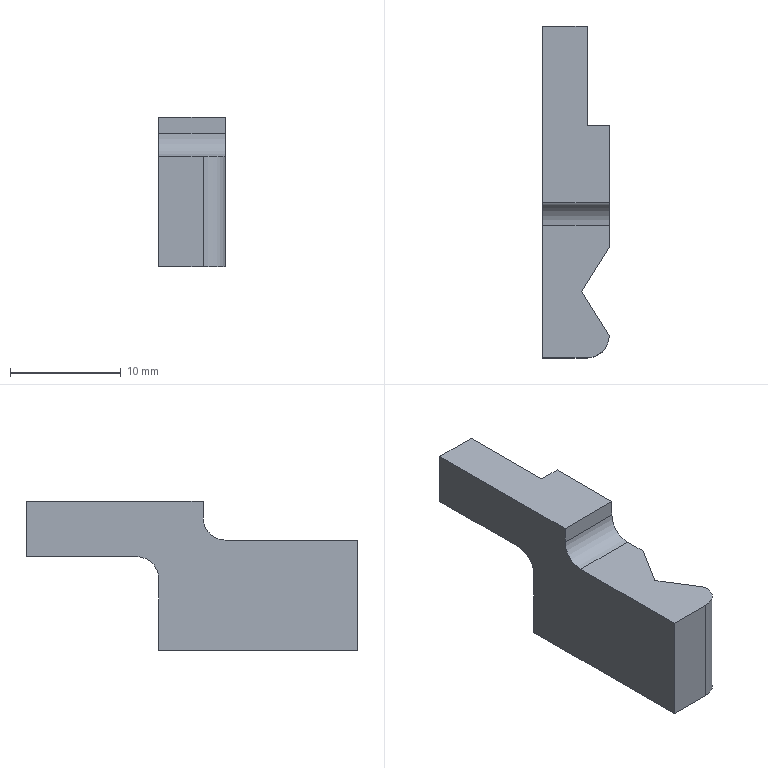Part | STEP file | 2012-06-08-012 | 1 solid | 17 faces | box 6 x 30 x 13.5 mm | volume 1336 mm3 | plane 14 | cylinder 3 | commonest cylinder face diameters 4 x3
STEP:
#1=CARTESIAN_POINT('',(0.,0.,0.));
#2=DIRECTION('',(0.,0.,1.));
#3=DIRECTION('',(1.,0.,0.));
#4=AXIS2_PLACEMENT_3D('',#1,#2,#3);
#5=CARTESIAN_POINT('',(0.,0.,10.));
#6=VERTEX_POINT('',#5);
#7=CARTESIAN_POINT('',(0.,12.,10.));
#8=VERTEX_POINT('',#7);
#9=CARTESIAN_POINT('',(0.,0.,10.));
#10=DIRECTION('',(0.,1.,0.));
#11=VECTOR('',#10,1.);
#12=LINE('',#9,#11);
#13=CARTESIAN_POINT('',(0.,0.,13.5));
#14=DIRECTION('',(1.,0.,0.));
#15=DIRECTION('',(0.,0.,-1.));
#16=AXIS2_PLACEMENT_3D('',#13,#14,#15);
#17=PLANE('',#16);
#18=CARTESIAN_POINT('',(3.5,0.));
#19=DIRECTION('',(0.,1.));
#20=VECTOR('',#19,1.);
#21=LINE('',#18,#20);
#22=(GEOMETRIC_REPRESENTATION_CONTEXT(2)PARAMETRIC_REPRESENTATION_CONTEXT()REPRESENTATION_CONTEXT('',''));
#23=DEFINITIONAL_REPRESENTATION('',(#21),#22);
#24=PCURVE('',#17,#23);
#25=CARTESIAN_POINT('',(-4.,14.,10.));
#26=DIRECTION('',(0.,0.,-1.));
#27=DIRECTION('',(0.,1.,0.));
#28=AXIS2_PLACEMENT_3D('',#25,#26,#27);
#29=PLANE('',#28);
#30=CARTESIAN_POINT('',(-14.,4.));
#31=DIRECTION('',(1.,0.));
#32=VECTOR('',#31,1.);
#33=LINE('',#30,#32);
#34=(GEOMETRIC_REPRESENTATION_CONTEXT(2)PARAMETRIC_REPRESENTATION_CONTEXT()REPRESENTATION_CONTEXT('',''));
#35=DEFINITIONAL_REPRESENTATION('',(#33),#34);
#36=PCURVE('',#29,#35);
#37=SURFACE_CURVE('',#12,(#24,#36),.PCURVE_S1.);
#38=EDGE_CURVE('',#6,#8,#37,.T.);
#39=ORIENTED_EDGE('',*,*,#38,.T.);
#40=CARTESIAN_POINT('',(0.,14.,12.));
#41=VERTEX_POINT('',#40);
#42=CARTESIAN_POINT('',(0.,12.,12.));
#43=DIRECTION('',(1.,0.,0.));
#44=DIRECTION('',(0.,0.,-1.));
#45=AXIS2_PLACEMENT_3D('',#42,#43,#44);
#46=CIRCLE('',#45,2.);
#47=CARTESIAN_POINT('',(1.5,12.));
#48=DIRECTION('',(1.,0.));
#49=AXIS2_PLACEMENT_2D('',#47,#48);
#50=CIRCLE('',#49,2.);
#51=(GEOMETRIC_REPRESENTATION_CONTEXT(2)PARAMETRIC_REPRESENTATION_CONTEXT()REPRESENTATION_CONTEXT('',''));
#52=DEFINITIONAL_REPRESENTATION('',(#50),#51);
#53=PCURVE('',#17,#52);
#54=CARTESIAN_POINT('',(-4.,12.,12.));
#55=DIRECTION('',(-1.,0.,0.));
#56=DIRECTION('',(0.,0.,1.));
#57=AXIS2_PLACEMENT_3D('',#54,#55,#56);
#58=CYLINDRICAL_SURFACE('',#57,2.);
#59=CARTESIAN_POINT('',(3.142,-4.));
#60=DIRECTION('',(-1.,0.));
#61=VECTOR('',#60,1.);
#62=LINE('',#59,#61);
#63=(GEOMETRIC_REPRESENTATION_CONTEXT(2)PARAMETRIC_REPRESENTATION_CONTEXT()REPRESENTATION_CONTEXT('',''));
#64=DEFINITIONAL_REPRESENTATION('',(#62),#63);
#65=PCURVE('',#58,#64);
#66=SURFACE_CURVE('',#46,(#53,#65),.PCURVE_S1.);
#67=EDGE_CURVE('',#8,#41,#66,.T.);
#68=ORIENTED_EDGE('',*,*,#67,.T.);
#69=CARTESIAN_POINT('',(0.,14.,13.5));
#70=VERTEX_POINT('',#69);
#71=CARTESIAN_POINT('',(0.,14.,13.5));
#72=DIRECTION('',(0.,0.,1.));
#73=VECTOR('',#72,1.);
#74=LINE('',#71,#73);
#75=CARTESIAN_POINT('',(0.,14.));
#76=DIRECTION('',(-1.,0.));
#77=VECTOR('',#76,1.);
#78=LINE('',#75,#77);
#79=(GEOMETRIC_REPRESENTATION_CONTEXT(2)PARAMETRIC_REPRESENTATION_CONTEXT()REPRESENTATION_CONTEXT('',''));
#80=DEFINITIONAL_REPRESENTATION('',(#78),#79);
#81=PCURVE('',#17,#80);
#82=CARTESIAN_POINT('',(-4.,14.,13.5));
#83=DIRECTION('',(0.,1.,0.));
#84=DIRECTION('',(0.,0.,1.));
#85=AXIS2_PLACEMENT_3D('',#82,#83,#84);
#86=PLANE('',#85);
#87=CARTESIAN_POINT('',(0.,4.));
#88=DIRECTION('',(1.,0.));
#89=VECTOR('',#88,1.);
#90=LINE('',#87,#89);
#91=(GEOMETRIC_REPRESENTATION_CONTEXT(2)PARAMETRIC_REPRESENTATION_CONTEXT()REPRESENTATION_CONTEXT('',''));
#92=DEFINITIONAL_REPRESENTATION('',(#90),#91);
#93=PCURVE('',#86,#92);
#94=SURFACE_CURVE('',#74,(#81,#93),.PCURVE_S1.);
#95=EDGE_CURVE('',#41,#70,#94,.T.);
#96=ORIENTED_EDGE('',*,*,#95,.T.);
#97=CARTESIAN_POINT('',(0.,30.,13.5));
#98=VERTEX_POINT('',#97);
#99=CARTESIAN_POINT('',(0.,0.,13.5));
#100=DIRECTION('',(0.,-1.,0.));
#101=VECTOR('',#100,1.);
#102=LINE('',#99,#101);
#103=CARTESIAN_POINT('',(0.,0.));
#104=DIRECTION('',(0.,-1.));
#105=VECTOR('',#104,1.);
#106=LINE('',#103,#105);
#107=(GEOMETRIC_REPRESENTATION_CONTEXT(2)PARAMETRIC_REPRESENTATION_CONTEXT()REPRESENTATION_CONTEXT('',''));
#108=DEFINITIONAL_REPRESENTATION('',(#106),#107);
#109=PCURVE('',#17,#108);
#110=CARTESIAN_POINT('',(0.,30.,13.5));
#111=DIRECTION('',(0.,0.,-1.));
#112=DIRECTION('',(-1.,0.,0.));
#113=AXIS2_PLACEMENT_3D('',#110,#111,#112);
#114=PLANE('',#113);
#115=CARTESIAN_POINT('',(0.,-30.));
#116=DIRECTION('',(0.,-1.));
#117=VECTOR('',#116,1.);
#118=LINE('',#115,#117);
#119=(GEOMETRIC_REPRESENTATION_CONTEXT(2)PARAMETRIC_REPRESENTATION_CONTEXT()REPRESENTATION_CONTEXT('',''));
#120=DEFINITIONAL_REPRESENTATION('',(#118),#119);
#121=PCURVE('',#114,#120);
#122=SURFACE_CURVE('',#102,(#109,#121),.PCURVE_S1.);
#123=EDGE_CURVE('',#98,#70,#122,.T.);
#124=ORIENTED_EDGE('',*,*,#123,.F.);
#125=CARTESIAN_POINT('',(0.,30.,8.5));
#126=VERTEX_POINT('',#125);
#127=CARTESIAN_POINT('',(0.,30.,13.5));
#128=DIRECTION('',(0.,0.,-1.));
#129=VECTOR('',#128,1.);
#130=LINE('',#127,#129);
#131=CARTESIAN_POINT('',(0.,30.));
#132=DIRECTION('',(1.,0.));
#133=VECTOR('',#132,1.);
#134=LINE('',#131,#133);
#135=(GEOMETRIC_REPRESENTATION_CONTEXT(2)PARAMETRIC_REPRESENTATION_CONTEXT()REPRESENTATION_CONTEXT('',''));
#136=DEFINITIONAL_REPRESENTATION('',(#134),#135);
#137=PCURVE('',#17,#136);
#138=CARTESIAN_POINT('',(0.,30.,13.5));
#139=DIRECTION('',(0.,-1.,0.));
#140=DIRECTION('',(0.,0.,-1.));
#141=AXIS2_PLACEMENT_3D('',#138,#139,#140);
#142=PLANE('',#141);
#143=CARTESIAN_POINT('',(0.,0.));
#144=DIRECTION('',(1.,0.));
#145=VECTOR('',#144,1.);
#146=LINE('',#143,#145);
#147=(GEOMETRIC_REPRESENTATION_CONTEXT(2)PARAMETRIC_REPRESENTATION_CONTEXT()REPRESENTATION_CONTEXT('',''));
#148=DEFINITIONAL_REPRESENTATION('',(#146),#147);
#149=PCURVE('',#142,#148);
#150=SURFACE_CURVE('',#130,(#137,#149),.PCURVE_S1.);
#151=EDGE_CURVE('',#98,#126,#150,.T.);
#152=ORIENTED_EDGE('',*,*,#151,.T.);
#153=CARTESIAN_POINT('',(0.,20.,8.5));
#154=VERTEX_POINT('',#153);
#155=CARTESIAN_POINT('',(0.,0.,8.5));
#156=DIRECTION('',(0.,-1.,0.));
#157=VECTOR('',#156,1.);
#158=LINE('',#155,#157);
#159=CARTESIAN_POINT('',(5.,0.));
#160=DIRECTION('',(0.,-1.));
#161=VECTOR('',#160,1.);
#162=LINE('',#159,#161);
#163=(GEOMETRIC_REPRESENTATION_CONTEXT(2)PARAMETRIC_REPRESENTATION_CONTEXT()REPRESENTATION_CONTEXT('',''));
#164=DEFINITIONAL_REPRESENTATION('',(#162),#163);
#165=PCURVE('',#17,#164);
#166=CARTESIAN_POINT('',(-4.,30.,8.5));
#167=DIRECTION('',(0.,0.,1.));
#168=DIRECTION('',(0.,-1.,0.));
#169=AXIS2_PLACEMENT_3D('',#166,#167,#168);
#170=PLANE('',#169);
#171=CARTESIAN_POINT('',(30.,4.));
#172=DIRECTION('',(1.,0.));
#173=VECTOR('',#172,1.);
#174=LINE('',#171,#173);
#175=(GEOMETRIC_REPRESENTATION_CONTEXT(2)PARAMETRIC_REPRESENTATION_CONTEXT()REPRESENTATION_CONTEXT('',''));
#176=DEFINITIONAL_REPRESENTATION('',(#174),#175);
#177=PCURVE('',#170,#176);
#178=SURFACE_CURVE('',#158,(#165,#177),.PCURVE_S1.);
#179=EDGE_CURVE('',#126,#154,#178,.T.);
#180=ORIENTED_EDGE('',*,*,#179,.T.);
#181=CARTESIAN_POINT('',(0.,18.,6.5));
#182=VERTEX_POINT('',#181);
#183=CARTESIAN_POINT('',(0.,20.,6.5));
#184=DIRECTION('',(1.,0.,0.));
#185=DIRECTION('',(0.,0.,-1.));
#186=AXIS2_PLACEMENT_3D('',#183,#184,#185);
#187=CIRCLE('',#186,2.);
#188=CARTESIAN_POINT('',(7.,20.));
#189=DIRECTION('',(1.,0.));
#190=AXIS2_PLACEMENT_2D('',#188,#189);
#191=CIRCLE('',#190,2.);
#192=(GEOMETRIC_REPRESENTATION_CONTEXT(2)PARAMETRIC_REPRESENTATION_CONTEXT()REPRESENTATION_CONTEXT('',''));
#193=DEFINITIONAL_REPRESENTATION('',(#191),#192);
#194=PCURVE('',#17,#193);
#195=CARTESIAN_POINT('',(-4.,20.,6.5));
#196=DIRECTION('',(-1.,0.,0.));
#197=DIRECTION('',(0.,0.,1.));
#198=AXIS2_PLACEMENT_3D('',#195,#196,#197);
#199=CYLINDRICAL_SURFACE('',#198,2.);
#200=CARTESIAN_POINT('',(9.425,-4.));
#201=DIRECTION('',(-1.,0.));
#202=VECTOR('',#201,1.);
#203=LINE('',#200,#202);
#204=(GEOMETRIC_REPRESENTATION_CONTEXT(2)PARAMETRIC_REPRESENTATION_CONTEXT()REPRESENTATION_CONTEXT('',''));
#205=DEFINITIONAL_REPRESENTATION('',(#203),#204);
#206=PCURVE('',#199,#205);
#207=SURFACE_CURVE('',#187,(#194,#206),.PCURVE_S1.);
#208=EDGE_CURVE('',#154,#182,#207,.T.);
#209=ORIENTED_EDGE('',*,*,#208,.T.);
#210=CARTESIAN_POINT('',(0.,18.,0.));
#211=VERTEX_POINT('',#210);
#212=CARTESIAN_POINT('',(0.,18.,13.5));
#213=DIRECTION('',(0.,0.,-1.));
#214=VECTOR('',#213,1.);
#215=LINE('',#212,#214);
#216=CARTESIAN_POINT('',(0.,18.));
#217=DIRECTION('',(1.,0.));
#218=VECTOR('',#217,1.);
#219=LINE('',#216,#218);
#220=(GEOMETRIC_REPRESENTATION_CONTEXT(2)PARAMETRIC_REPRESENTATION_CONTEXT()REPRESENTATION_CONTEXT('',''));
#221=DEFINITIONAL_REPRESENTATION('',(#219),#220);
#222=PCURVE('',#17,#221);
#223=CARTESIAN_POINT('',(-4.,18.,0.));
#224=DIRECTION('',(0.,-1.,0.));
#225=DIRECTION('',(0.,0.,-1.));
#226=AXIS2_PLACEMENT_3D('',#223,#224,#225);
#227=PLANE('',#226);
#228=CARTESIAN_POINT('',(-13.5,4.));
#229=DIRECTION('',(1.,0.));
#230=VECTOR('',#229,1.);
#231=LINE('',#228,#230);
#232=(GEOMETRIC_REPRESENTATION_CONTEXT(2)PARAMETRIC_REPRESENTATION_CONTEXT()REPRESENTATION_CONTEXT('',''));
#233=DEFINITIONAL_REPRESENTATION('',(#231),#232);
#234=PCURVE('',#227,#233);
#235=SURFACE_CURVE('',#215,(#222,#234),.PCURVE_S1.);
#236=EDGE_CURVE('',#182,#211,#235,.T.);
#237=ORIENTED_EDGE('',*,*,#236,.T.);
#238=CARTESIAN_POINT('',(0.,0.,0.));
#239=VERTEX_POINT('',#238);
#240=CARTESIAN_POINT('',(0.,0.,0.));
#241=DIRECTION('',(0.,-1.,0.));
#242=VECTOR('',#241,1.);
#243=LINE('',#240,#242);
#244=CARTESIAN_POINT('',(13.5,0.));
#245=DIRECTION('',(0.,-1.));
#246=VECTOR('',#245,1.);
#247=LINE('',#244,#246);
#248=(GEOMETRIC_REPRESENTATION_CONTEXT(2)PARAMETRIC_REPRESENTATION_CONTEXT()REPRESENTATION_CONTEXT('',''));
#249=DEFINITIONAL_REPRESENTATION('',(#247),#248);
#250=PCURVE('',#17,#249);
#251=CARTESIAN_POINT('',(0.,30.,0.));
#252=DIRECTION('',(0.,0.,-1.));
#253=DIRECTION('',(-1.,0.,0.));
#254=AXIS2_PLACEMENT_3D('',#251,#252,#253);
#255=PLANE('',#254);
#256=CARTESIAN_POINT('',(0.,-30.));
#257=DIRECTION('',(0.,-1.));
#258=VECTOR('',#257,1.);
#259=LINE('',#256,#258);
#260=(GEOMETRIC_REPRESENTATION_CONTEXT(2)PARAMETRIC_REPRESENTATION_CONTEXT()REPRESENTATION_CONTEXT('',''));
#261=DEFINITIONAL_REPRESENTATION('',(#259),#260);
#262=PCURVE('',#255,#261);
#263=SURFACE_CURVE('',#243,(#250,#262),.PCURVE_S1.);
#264=EDGE_CURVE('',#211,#239,#263,.T.);
#265=ORIENTED_EDGE('',*,*,#264,.T.);
#266=CARTESIAN_POINT('',(0.,0.,13.5));
#267=DIRECTION('',(0.,0.,-1.));
#268=VECTOR('',#267,1.);
#269=LINE('',#266,#268);
#270=CARTESIAN_POINT('',(0.,0.));
#271=DIRECTION('',(1.,0.));
#272=VECTOR('',#271,1.);
#273=LINE('',#270,#272);
#274=(GEOMETRIC_REPRESENTATION_CONTEXT(2)PARAMETRIC_REPRESENTATION_CONTEXT()REPRESENTATION_CONTEXT('',''));
#275=DEFINITIONAL_REPRESENTATION('',(#273),#274);
#276=PCURVE('',#17,#275);
#277=CARTESIAN_POINT('',(0.,0.,13.5));
#278=DIRECTION('',(0.,1.,0.));
#279=DIRECTION('',(0.,0.,1.));
#280=AXIS2_PLACEMENT_3D('',#277,#278,#279);
#281=PLANE('',#280);
#282=CARTESIAN_POINT('',(0.,0.));
#283=DIRECTION('',(-1.,0.));
#284=VECTOR('',#283,1.);
#285=LINE('',#282,#284);
#286=(GEOMETRIC_REPRESENTATION_CONTEXT(2)PARAMETRIC_REPRESENTATION_CONTEXT()REPRESENTATION_CONTEXT('',''));
#287=DEFINITIONAL_REPRESENTATION('',(#285),#286);
#288=PCURVE('',#281,#287);
#289=SURFACE_CURVE('',#269,(#276,#288),.PCURVE_S1.);
#290=EDGE_CURVE('',#6,#239,#289,.T.);
#291=ORIENTED_EDGE('',*,*,#290,.F.);
#292=EDGE_LOOP('',(#39,#68,#96,#124,#152,#180,#209,#237,#265,#291));
#293=FACE_BOUND('',#292,.T.);
#294=ADVANCED_FACE('',(#293),#17,.F.);
#295=CARTESIAN_POINT('',(4.,0.,0.));
#296=VERTEX_POINT('',#295);
#297=CARTESIAN_POINT('',(4.,0.,10.));
#298=VERTEX_POINT('',#297);
#299=CARTESIAN_POINT('',(4.,0.,13.5));
#300=DIRECTION('',(0.,0.,1.));
#301=VECTOR('',#300,1.);
#302=LINE('',#299,#301);
#303=CARTESIAN_POINT('',(0.,4.));
#304=DIRECTION('',(1.,0.));
#305=VECTOR('',#304,1.);
#306=LINE('',#303,#305);
#307=(GEOMETRIC_REPRESENTATION_CONTEXT(2)PARAMETRIC_REPRESENTATION_CONTEXT()REPRESENTATION_CONTEXT('',''));
#308=DEFINITIONAL_REPRESENTATION('',(#306),#307);
#309=PCURVE('',#281,#308);
#310=CARTESIAN_POINT('',(4.,2.,13.5));
#311=DIRECTION('',(0.,0.,-1.));
#312=DIRECTION('',(-1.,0.,0.));
#313=AXIS2_PLACEMENT_3D('',#310,#311,#312);
#314=CYLINDRICAL_SURFACE('',#313,2.);
#315=CARTESIAN_POINT('',(4.712,0.));
#316=DIRECTION('',(0.,-1.));
#317=VECTOR('',#316,1.);
#318=LINE('',#315,#317);
#319=(GEOMETRIC_REPRESENTATION_CONTEXT(2)PARAMETRIC_REPRESENTATION_CONTEXT()REPRESENTATION_CONTEXT('',''));
#320=DEFINITIONAL_REPRESENTATION('',(#318),#319);
#321=PCURVE('',#314,#320);
#322=SURFACE_CURVE('',#302,(#309,#321),.PCURVE_S1.);
#323=EDGE_CURVE('',#296,#298,#322,.T.);
#324=ORIENTED_EDGE('',*,*,#323,.T.);
#325=CARTESIAN_POINT('',(-4.,0.,10.));
#326=DIRECTION('',(1.,0.,0.));
#327=VECTOR('',#326,1.);
#328=LINE('',#325,#327);
#329=CARTESIAN_POINT('',(-3.5,-4.));
#330=DIRECTION('',(0.,1.));
#331=VECTOR('',#330,1.);
#332=LINE('',#329,#331);
#333=(GEOMETRIC_REPRESENTATION_CONTEXT(2)PARAMETRIC_REPRESENTATION_CONTEXT()REPRESENTATION_CONTEXT('',''));
#334=DEFINITIONAL_REPRESENTATION('',(#332),#333);
#335=PCURVE('',#281,#334);
#336=CARTESIAN_POINT('',(-14.,0.));
#337=DIRECTION('',(0.,1.));
#338=VECTOR('',#337,1.);
#339=LINE('',#336,#338);
#340=(GEOMETRIC_REPRESENTATION_CONTEXT(2)PARAMETRIC_REPRESENTATION_CONTEXT()REPRESENTATION_CONTEXT('',''));
#341=DEFINITIONAL_REPRESENTATION('',(#339),#340);
#342=PCURVE('',#29,#341);
#343=SURFACE_CURVE('',#328,(#335,#342),.PCURVE_S1.);
#344=EDGE_CURVE('',#6,#298,#343,.T.);
#345=ORIENTED_EDGE('',*,*,#344,.F.);
#346=ORIENTED_EDGE('',*,*,#290,.T.);
#347=CARTESIAN_POINT('',(0.,0.,0.));
#348=DIRECTION('',(1.,0.,0.));
#349=VECTOR('',#348,1.);
#350=LINE('',#347,#349);
#351=CARTESIAN_POINT('',(-13.5,0.));
#352=DIRECTION('',(0.,1.));
#353=VECTOR('',#352,1.);
#354=LINE('',#351,#353);
#355=(GEOMETRIC_REPRESENTATION_CONTEXT(2)PARAMETRIC_REPRESENTATION_CONTEXT()REPRESENTATION_CONTEXT('',''));
#356=DEFINITIONAL_REPRESENTATION('',(#354),#355);
#357=PCURVE('',#281,#356);
#358=CARTESIAN_POINT('',(0.,-30.));
#359=DIRECTION('',(-1.,0.));
#360=VECTOR('',#359,1.);
#361=LINE('',#358,#360);
#362=(GEOMETRIC_REPRESENTATION_CONTEXT(2)PARAMETRIC_REPRESENTATION_CONTEXT()REPRESENTATION_CONTEXT('',''));
#363=DEFINITIONAL_REPRESENTATION('',(#361),#362);
#364=PCURVE('',#255,#363);
#365=SURFACE_CURVE('',#350,(#357,#364),.PCURVE_S1.);
#366=EDGE_CURVE('',#239,#296,#365,.T.);
#367=ORIENTED_EDGE('',*,*,#366,.T.);
#368=EDGE_LOOP('',(#324,#345,#346,#367));
#369=FACE_BOUND('',#368,.T.);
#370=ADVANCED_FACE('',(#369),#281,.F.);
#371=CARTESIAN_POINT('',(3.5,6.,10.));
#372=VERTEX_POINT('',#371);
#373=CARTESIAN_POINT('',(3.5,6.,0.));
#374=VERTEX_POINT('',#373);
#375=CARTESIAN_POINT('',(3.5,6.,13.5));
#376=DIRECTION('',(0.,0.,-1.));
#377=VECTOR('',#376,1.);
#378=LINE('',#375,#377);
#379=CARTESIAN_POINT('',(3.5,6.,13.5));
#380=DIRECTION('',(-0.848,-0.53,0.));
#381=DIRECTION('',(0.53,-0.848,0.));
#382=AXIS2_PLACEMENT_3D('',#379,#380,#381);
#383=PLANE('',#382);
#384=CARTESIAN_POINT('',(0.,0.));
#385=DIRECTION('',(0.,-1.));
#386=VECTOR('',#385,1.);
#387=LINE('',#384,#386);
#388=(GEOMETRIC_REPRESENTATION_CONTEXT(2)PARAMETRIC_REPRESENTATION_CONTEXT()REPRESENTATION_CONTEXT('',''));
#389=DEFINITIONAL_REPRESENTATION('',(#387),#388);
#390=PCURVE('',#383,#389);
#391=CARTESIAN_POINT('',(6.,10.,13.5));
#392=DIRECTION('',(-0.848,0.53,0.));
#393=DIRECTION('',(-0.53,-0.848,0.));
#394=AXIS2_PLACEMENT_3D('',#391,#392,#393);
#395=PLANE('',#394);
#396=CARTESIAN_POINT('',(4.717,0.));
#397=DIRECTION('',(0.,-1.));
#398=VECTOR('',#397,1.);
#399=LINE('',#396,#398);
#400=(GEOMETRIC_REPRESENTATION_CONTEXT(2)PARAMETRIC_REPRESENTATION_CONTEXT()REPRESENTATION_CONTEXT('',''));
#401=DEFINITIONAL_REPRESENTATION('',(#399),#400);
#402=PCURVE('',#395,#401);
#403=SURFACE_CURVE('',#378,(#390,#402),.PCURVE_S1.);
#404=EDGE_CURVE('',#372,#374,#403,.T.);
#405=ORIENTED_EDGE('',*,*,#404,.F.);
#406=CARTESIAN_POINT('',(6.,2.,10.));
#407=VERTEX_POINT('',#406);
#408=CARTESIAN_POINT('',(3.5,6.,10.));
#409=DIRECTION('',(0.53,-0.848,0.));
#410=VECTOR('',#409,1.);
#411=LINE('',#408,#410);
#412=CARTESIAN_POINT('',(0.,-3.5));
#413=DIRECTION('',(1.,0.));
#414=VECTOR('',#413,1.);
#415=LINE('',#412,#414);
#416=(GEOMETRIC_REPRESENTATION_CONTEXT(2)PARAMETRIC_REPRESENTATION_CONTEXT()REPRESENTATION_CONTEXT('',''));
#417=DEFINITIONAL_REPRESENTATION('',(#415),#416);
#418=PCURVE('',#383,#417);
#419=CARTESIAN_POINT('',(-8.,7.5));
#420=DIRECTION('',(-0.848,0.53));
#421=VECTOR('',#420,1.);
#422=LINE('',#419,#421);
#423=(GEOMETRIC_REPRESENTATION_CONTEXT(2)PARAMETRIC_REPRESENTATION_CONTEXT()REPRESENTATION_CONTEXT('',''));
#424=DEFINITIONAL_REPRESENTATION('',(#422),#423);
#425=PCURVE('',#29,#424);
#426=SURFACE_CURVE('',#411,(#418,#425),.PCURVE_S1.);
#427=EDGE_CURVE('',#372,#407,#426,.T.);
#428=ORIENTED_EDGE('',*,*,#427,.T.);
#429=CARTESIAN_POINT('',(6.,2.,0.));
#430=VERTEX_POINT('',#429);
#431=CARTESIAN_POINT('',(6.,2.,13.5));
#432=DIRECTION('',(0.,0.,-1.));
#433=VECTOR('',#432,1.);
#434=LINE('',#431,#433);
#435=CARTESIAN_POINT('',(4.717,0.));
#436=DIRECTION('',(0.,-1.));
#437=VECTOR('',#436,1.);
#438=LINE('',#435,#437);
#439=(GEOMETRIC_REPRESENTATION_CONTEXT(2)PARAMETRIC_REPRESENTATION_CONTEXT()REPRESENTATION_CONTEXT('',''));
#440=DEFINITIONAL_REPRESENTATION('',(#438),#439);
#441=PCURVE('',#383,#440);
#442=CARTESIAN_POINT('',(3.142,0.));
#443=DIRECTION('',(0.,1.));
#444=VECTOR('',#443,1.);
#445=LINE('',#442,#444);
#446=(GEOMETRIC_REPRESENTATION_CONTEXT(2)PARAMETRIC_REPRESENTATION_CONTEXT()REPRESENTATION_CONTEXT('',''));
#447=DEFINITIONAL_REPRESENTATION('',(#445),#446);
#448=PCURVE('',#314,#447);
#449=SURFACE_CURVE('',#434,(#441,#448),.PCURVE_S1.);
#450=EDGE_CURVE('',#407,#430,#449,.T.);
#451=ORIENTED_EDGE('',*,*,#450,.T.);
#452=CARTESIAN_POINT('',(3.5,6.,0.));
#453=DIRECTION('',(-0.53,0.848,0.));
#454=VECTOR('',#453,1.);
#455=LINE('',#452,#454);
#456=CARTESIAN_POINT('',(0.,-13.5));
#457=DIRECTION('',(-1.,0.));
#458=VECTOR('',#457,1.);
#459=LINE('',#456,#458);
#460=(GEOMETRIC_REPRESENTATION_CONTEXT(2)PARAMETRIC_REPRESENTATION_CONTEXT()REPRESENTATION_CONTEXT('',''));
#461=DEFINITIONAL_REPRESENTATION('',(#459),#460);
#462=PCURVE('',#383,#461);
#463=CARTESIAN_POINT('',(-3.5,-24.));
#464=DIRECTION('',(0.53,0.848));
#465=VECTOR('',#464,1.);
#466=LINE('',#463,#465);
#467=(GEOMETRIC_REPRESENTATION_CONTEXT(2)PARAMETRIC_REPRESENTATION_CONTEXT()REPRESENTATION_CONTEXT('',''));
#468=DEFINITIONAL_REPRESENTATION('',(#466),#467);
#469=PCURVE('',#255,#468);
#470=SURFACE_CURVE('',#455,(#462,#469),.PCURVE_S1.);
#471=EDGE_CURVE('',#430,#374,#470,.T.);
#472=ORIENTED_EDGE('',*,*,#471,.T.);
#473=EDGE_LOOP('',(#405,#428,#451,#472));
#474=FACE_BOUND('',#473,.T.);
#475=ADVANCED_FACE('',(#474),#383,.F.);
#476=CARTESIAN_POINT('',(6.,10.,10.));
#477=VERTEX_POINT('',#476);
#478=CARTESIAN_POINT('',(6.,10.,0.));
#479=VERTEX_POINT('',#478);
#480=CARTESIAN_POINT('',(6.,10.,13.5));
#481=DIRECTION('',(0.,0.,-1.));
#482=VECTOR('',#481,1.);
#483=LINE('',#480,#482);
#484=CARTESIAN_POINT('',(0.,0.));
#485=DIRECTION('',(0.,-1.));
#486=VECTOR('',#485,1.);
#487=LINE('',#484,#486);
#488=(GEOMETRIC_REPRESENTATION_CONTEXT(2)PARAMETRIC_REPRESENTATION_CONTEXT()REPRESENTATION_CONTEXT('',''));
#489=DEFINITIONAL_REPRESENTATION('',(#487),#488);
#490=PCURVE('',#395,#489);
#491=CARTESIAN_POINT('',(6.,10.,13.5));
#492=DIRECTION('',(-1.,0.,0.));
#493=DIRECTION('',(0.,0.,1.));
#494=AXIS2_PLACEMENT_3D('',#491,#492,#493);
#495=PLANE('',#494);
#496=CARTESIAN_POINT('',(0.,0.));
#497=DIRECTION('',(-1.,0.));
#498=VECTOR('',#497,1.);
#499=LINE('',#496,#498);
#500=(GEOMETRIC_REPRESENTATION_CONTEXT(2)PARAMETRIC_REPRESENTATION_CONTEXT()REPRESENTATION_CONTEXT('',''));
#501=DEFINITIONAL_REPRESENTATION('',(#499),#500);
#502=PCURVE('',#495,#501);
#503=SURFACE_CURVE('',#483,(#490,#502),.PCURVE_S1.);
#504=EDGE_CURVE('',#477,#479,#503,.T.);
#505=ORIENTED_EDGE('',*,*,#504,.F.);
#506=CARTESIAN_POINT('',(6.,10.,10.));
#507=DIRECTION('',(-0.53,-0.848,0.));
#508=VECTOR('',#507,1.);
#509=LINE('',#506,#508);
#510=CARTESIAN_POINT('',(0.,-3.5));
#511=DIRECTION('',(1.,0.));
#512=VECTOR('',#511,1.);
#513=LINE('',#510,#512);
#514=(GEOMETRIC_REPRESENTATION_CONTEXT(2)PARAMETRIC_REPRESENTATION_CONTEXT()REPRESENTATION_CONTEXT('',''));
#515=DEFINITIONAL_REPRESENTATION('',(#513),#514);
#516=PCURVE('',#395,#515);
#517=CARTESIAN_POINT('',(-4.,10.));
#518=DIRECTION('',(-0.848,-0.53));
#519=VECTOR('',#518,1.);
#520=LINE('',#517,#519);
#521=(GEOMETRIC_REPRESENTATION_CONTEXT(2)PARAMETRIC_REPRESENTATION_CONTEXT()REPRESENTATION_CONTEXT('',''));
#522=DEFINITIONAL_REPRESENTATION('',(#520),#521);
#523=PCURVE('',#29,#522);
#524=SURFACE_CURVE('',#509,(#516,#523),.PCURVE_S1.);
#525=EDGE_CURVE('',#477,#372,#524,.T.);
#526=ORIENTED_EDGE('',*,*,#525,.T.);
#527=ORIENTED_EDGE('',*,*,#404,.T.);
#528=CARTESIAN_POINT('',(6.,10.,0.));
#529=DIRECTION('',(0.53,0.848,0.));
#530=VECTOR('',#529,1.);
#531=LINE('',#528,#530);
#532=CARTESIAN_POINT('',(0.,-13.5));
#533=DIRECTION('',(-1.,0.));
#534=VECTOR('',#533,1.);
#535=LINE('',#532,#534);
#536=(GEOMETRIC_REPRESENTATION_CONTEXT(2)PARAMETRIC_REPRESENTATION_CONTEXT()REPRESENTATION_CONTEXT('',''));
#537=DEFINITIONAL_REPRESENTATION('',(#535),#536);
#538=PCURVE('',#395,#537);
#539=CARTESIAN_POINT('',(-6.,-20.));
#540=DIRECTION('',(-0.53,0.848));
#541=VECTOR('',#540,1.);
#542=LINE('',#539,#541);
#543=(GEOMETRIC_REPRESENTATION_CONTEXT(2)PARAMETRIC_REPRESENTATION_CONTEXT()REPRESENTATION_CONTEXT('',''));
#544=DEFINITIONAL_REPRESENTATION('',(#542),#543);
#545=PCURVE('',#255,#544);
#546=SURFACE_CURVE('',#531,(#538,#545),.PCURVE_S1.);
#547=EDGE_CURVE('',#374,#479,#546,.T.);
#548=ORIENTED_EDGE('',*,*,#547,.T.);
#549=EDGE_LOOP('',(#505,#526,#527,#548));
#550=FACE_BOUND('',#549,.T.);
#551=ADVANCED_FACE('',(#550),#395,.F.);
#552=CARTESIAN_POINT('',(6.,14.,13.5));
#553=VERTEX_POINT('',#552);
#554=CARTESIAN_POINT('',(6.,21.,13.5));
#555=VERTEX_POINT('',#554);
#556=CARTESIAN_POINT('',(6.,10.,13.5));
#557=DIRECTION('',(0.,1.,0.));
#558=VECTOR('',#557,1.);
#559=LINE('',#556,#558);
#560=CARTESIAN_POINT('',(0.,0.));
#561=DIRECTION('',(0.,1.));
#562=VECTOR('',#561,1.);
#563=LINE('',#560,#562);
#564=(GEOMETRIC_REPRESENTATION_CONTEXT(2)PARAMETRIC_REPRESENTATION_CONTEXT()REPRESENTATION_CONTEXT('',''));
#565=DEFINITIONAL_REPRESENTATION('',(#563),#564);
#566=PCURVE('',#495,#565);
#567=CARTESIAN_POINT('',(-6.,-20.));
#568=DIRECTION('',(0.,1.));
#569=VECTOR('',#568,1.);
#570=LINE('',#567,#569);
#571=(GEOMETRIC_REPRESENTATION_CONTEXT(2)PARAMETRIC_REPRESENTATION_CONTEXT()REPRESENTATION_CONTEXT('',''));
#572=DEFINITIONAL_REPRESENTATION('',(#570),#571);
#573=PCURVE('',#114,#572);
#574=SURFACE_CURVE('',#559,(#566,#573),.PCURVE_S1.);
#575=EDGE_CURVE('',#553,#555,#574,.T.);
#576=ORIENTED_EDGE('',*,*,#575,.F.);
#577=CARTESIAN_POINT('',(6.,14.,12.));
#578=VERTEX_POINT('',#577);
#579=CARTESIAN_POINT('',(6.,14.,13.5));
#580=DIRECTION('',(0.,0.,1.));
#581=VECTOR('',#580,1.);
#582=LINE('',#579,#581);
#583=CARTESIAN_POINT('',(0.,4.));
#584=DIRECTION('',(1.,0.));
#585=VECTOR('',#584,1.);
#586=LINE('',#583,#585);
#587=(GEOMETRIC_REPRESENTATION_CONTEXT(2)PARAMETRIC_REPRESENTATION_CONTEXT()REPRESENTATION_CONTEXT('',''));
#588=DEFINITIONAL_REPRESENTATION('',(#586),#587);
#589=PCURVE('',#495,#588);
#590=CARTESIAN_POINT('',(0.,10.));
#591=DIRECTION('',(1.,0.));
#592=VECTOR('',#591,1.);
#593=LINE('',#590,#592);
#594=(GEOMETRIC_REPRESENTATION_CONTEXT(2)PARAMETRIC_REPRESENTATION_CONTEXT()REPRESENTATION_CONTEXT('',''));
#595=DEFINITIONAL_REPRESENTATION('',(#593),#594);
#596=PCURVE('',#86,#595);
#597=SURFACE_CURVE('',#582,(#589,#596),.PCURVE_S1.);
#598=EDGE_CURVE('',#578,#553,#597,.T.);
#599=ORIENTED_EDGE('',*,*,#598,.F.);
#600=CARTESIAN_POINT('',(6.,12.,10.));
#601=VERTEX_POINT('',#600);
#602=CARTESIAN_POINT('',(6.,12.,12.));
#603=DIRECTION('',(-1.,0.,0.));
#604=DIRECTION('',(0.,0.,1.));
#605=AXIS2_PLACEMENT_3D('',#602,#603,#604);
#606=CIRCLE('',#605,2.);
#607=CARTESIAN_POINT('',(-1.5,2.));
#608=DIRECTION('',(1.,0.));
#609=AXIS2_PLACEMENT_2D('',#607,#608);
#610=CIRCLE('',#609,2.);
#611=(GEOMETRIC_REPRESENTATION_CONTEXT(2)PARAMETRIC_REPRESENTATION_CONTEXT()REPRESENTATION_CONTEXT('',''));
#612=DEFINITIONAL_REPRESENTATION('',(#610),#611);
#613=PCURVE('',#495,#612);
#614=CARTESIAN_POINT('',(0.,-10.));
#615=DIRECTION('',(1.,0.));
#616=VECTOR('',#615,1.);
#617=LINE('',#614,#616);
#618=(GEOMETRIC_REPRESENTATION_CONTEXT(2)PARAMETRIC_REPRESENTATION_CONTEXT()REPRESENTATION_CONTEXT('',''));
#619=DEFINITIONAL_REPRESENTATION('',(#617),#618);
#620=PCURVE('',#58,#619);
#621=SURFACE_CURVE('',#606,(#613,#620),.PCURVE_S1.);
#622=EDGE_CURVE('',#578,#601,#621,.T.);
#623=ORIENTED_EDGE('',*,*,#622,.T.);
#624=CARTESIAN_POINT('',(6.,14.,10.));
#625=DIRECTION('',(0.,1.,0.));
#626=VECTOR('',#625,1.);
#627=LINE('',#624,#626);
#628=CARTESIAN_POINT('',(-3.5,4.));
#629=DIRECTION('',(0.,1.));
#630=VECTOR('',#629,1.);
#631=LINE('',#628,#630);
#632=(GEOMETRIC_REPRESENTATION_CONTEXT(2)PARAMETRIC_REPRESENTATION_CONTEXT()REPRESENTATION_CONTEXT('',''));
#633=DEFINITIONAL_REPRESENTATION('',(#631),#632);
#634=PCURVE('',#495,#633);
#635=CARTESIAN_POINT('',(0.,10.));
#636=DIRECTION('',(1.,0.));
#637=VECTOR('',#636,1.);
#638=LINE('',#635,#637);
#639=(GEOMETRIC_REPRESENTATION_CONTEXT(2)PARAMETRIC_REPRESENTATION_CONTEXT()REPRESENTATION_CONTEXT('',''));
#640=DEFINITIONAL_REPRESENTATION('',(#638),#639);
#641=PCURVE('',#29,#640);
#642=SURFACE_CURVE('',#627,(#634,#641),.PCURVE_S1.);
#643=EDGE_CURVE('',#477,#601,#642,.T.);
#644=ORIENTED_EDGE('',*,*,#643,.F.);
#645=ORIENTED_EDGE('',*,*,#504,.T.);
#646=CARTESIAN_POINT('',(6.,18.,0.));
#647=VERTEX_POINT('',#646);
#648=CARTESIAN_POINT('',(6.,10.,0.));
#649=DIRECTION('',(0.,1.,0.));
#650=VECTOR('',#649,1.);
#651=LINE('',#648,#650);
#652=CARTESIAN_POINT('',(-13.5,0.));
#653=DIRECTION('',(0.,1.));
#654=VECTOR('',#653,1.);
#655=LINE('',#652,#654);
#656=(GEOMETRIC_REPRESENTATION_CONTEXT(2)PARAMETRIC_REPRESENTATION_CONTEXT()REPRESENTATION_CONTEXT('',''));
#657=DEFINITIONAL_REPRESENTATION('',(#655),#656);
#658=PCURVE('',#495,#657);
#659=CARTESIAN_POINT('',(-6.,-20.));
#660=DIRECTION('',(0.,1.));
#661=VECTOR('',#660,1.);
#662=LINE('',#659,#661);
#663=(GEOMETRIC_REPRESENTATION_CONTEXT(2)PARAMETRIC_REPRESENTATION_CONTEXT()REPRESENTATION_CONTEXT('',''));
#664=DEFINITIONAL_REPRESENTATION('',(#662),#663);
#665=PCURVE('',#255,#664);
#666=SURFACE_CURVE('',#651,(#658,#665),.PCURVE_S1.);
#667=EDGE_CURVE('',#479,#647,#666,.T.);
#668=ORIENTED_EDGE('',*,*,#667,.T.);
#669=CARTESIAN_POINT('',(6.,18.,6.5));
#670=VERTEX_POINT('',#669);
#671=CARTESIAN_POINT('',(6.,18.,0.));
#672=DIRECTION('',(0.,0.,-1.));
#673=VECTOR('',#672,1.);
#674=LINE('',#671,#673);
#675=CARTESIAN_POINT('',(-13.5,8.));
#676=DIRECTION('',(-1.,0.));
#677=VECTOR('',#676,1.);
#678=LINE('',#675,#677);
#679=(GEOMETRIC_REPRESENTATION_CONTEXT(2)PARAMETRIC_REPRESENTATION_CONTEXT()REPRESENTATION_CONTEXT('',''));
#680=DEFINITIONAL_REPRESENTATION('',(#678),#679);
#681=PCURVE('',#495,#680);
#682=CARTESIAN_POINT('',(0.,10.));
#683=DIRECTION('',(1.,0.));
#684=VECTOR('',#683,1.);
#685=LINE('',#682,#684);
#686=(GEOMETRIC_REPRESENTATION_CONTEXT(2)PARAMETRIC_REPRESENTATION_CONTEXT()REPRESENTATION_CONTEXT('',''));
#687=DEFINITIONAL_REPRESENTATION('',(#685),#686);
#688=PCURVE('',#227,#687);
#689=SURFACE_CURVE('',#674,(#681,#688),.PCURVE_S1.);
#690=EDGE_CURVE('',#670,#647,#689,.T.);
#691=ORIENTED_EDGE('',*,*,#690,.F.);
#692=CARTESIAN_POINT('',(6.,20.,8.5));
#693=VERTEX_POINT('',#692);
#694=CARTESIAN_POINT('',(6.,20.,6.5));
#695=DIRECTION('',(-1.,0.,0.));
#696=DIRECTION('',(0.,0.,1.));
#697=AXIS2_PLACEMENT_3D('',#694,#695,#696);
#698=CIRCLE('',#697,2.);
#699=CARTESIAN_POINT('',(-7.,10.));
#700=DIRECTION('',(1.,0.));
#701=AXIS2_PLACEMENT_2D('',#699,#700);
#702=CIRCLE('',#701,2.);
#703=(GEOMETRIC_REPRESENTATION_CONTEXT(2)PARAMETRIC_REPRESENTATION_CONTEXT()REPRESENTATION_CONTEXT('',''));
#704=DEFINITIONAL_REPRESENTATION('',(#702),#703);
#705=PCURVE('',#495,#704);
#706=CARTESIAN_POINT('',(0.,-10.));
#707=DIRECTION('',(1.,0.));
#708=VECTOR('',#707,1.);
#709=LINE('',#706,#708);
#710=(GEOMETRIC_REPRESENTATION_CONTEXT(2)PARAMETRIC_REPRESENTATION_CONTEXT()REPRESENTATION_CONTEXT('',''));
#711=DEFINITIONAL_REPRESENTATION('',(#709),#710);
#712=PCURVE('',#199,#711);
#713=SURFACE_CURVE('',#698,(#705,#712),.PCURVE_S1.);
#714=EDGE_CURVE('',#670,#693,#713,.T.);
#715=ORIENTED_EDGE('',*,*,#714,.T.);
#716=CARTESIAN_POINT('',(6.,21.,8.5));
#717=VERTEX_POINT('',#716);
#718=CARTESIAN_POINT('',(6.,30.,8.5));
#719=DIRECTION('',(0.,-1.,0.));
#720=VECTOR('',#719,1.);
#721=LINE('',#718,#720);
#722=CARTESIAN_POINT('',(-5.,20.));
#723=DIRECTION('',(0.,-1.));
#724=VECTOR('',#723,1.);
#725=LINE('',#722,#724);
#726=(GEOMETRIC_REPRESENTATION_CONTEXT(2)PARAMETRIC_REPRESENTATION_CONTEXT()REPRESENTATION_CONTEXT('',''));
#727=DEFINITIONAL_REPRESENTATION('',(#725),#726);
#728=PCURVE('',#495,#727);
#729=CARTESIAN_POINT('',(0.,10.));
#730=DIRECTION('',(1.,0.));
#731=VECTOR('',#730,1.);
#732=LINE('',#729,#731);
#733=(GEOMETRIC_REPRESENTATION_CONTEXT(2)PARAMETRIC_REPRESENTATION_CONTEXT()REPRESENTATION_CONTEXT('',''));
#734=DEFINITIONAL_REPRESENTATION('',(#732),#733);
#735=PCURVE('',#170,#734);
#736=SURFACE_CURVE('',#721,(#728,#735),.PCURVE_S1.);
#737=EDGE_CURVE('',#717,#693,#736,.T.);
#738=ORIENTED_EDGE('',*,*,#737,.F.);
#739=CARTESIAN_POINT('',(6.,21.,13.5));
#740=DIRECTION('',(0.,0.,-1.));
#741=VECTOR('',#740,1.);
#742=LINE('',#739,#741);
#743=CARTESIAN_POINT('',(0.,11.));
#744=DIRECTION('',(-1.,0.));
#745=VECTOR('',#744,1.);
#746=LINE('',#743,#745);
#747=(GEOMETRIC_REPRESENTATION_CONTEXT(2)PARAMETRIC_REPRESENTATION_CONTEXT()REPRESENTATION_CONTEXT('',''));
#748=DEFINITIONAL_REPRESENTATION('',(#746),#747);
#749=PCURVE('',#495,#748);
#750=CARTESIAN_POINT('',(4.,21.,13.5));
#751=DIRECTION('',(0.,-1.,0.));
#752=DIRECTION('',(0.,0.,-1.));
#753=AXIS2_PLACEMENT_3D('',#750,#751,#752);
#754=PLANE('',#753);
#755=CARTESIAN_POINT('',(0.,2.));
#756=DIRECTION('',(1.,0.));
#757=VECTOR('',#756,1.);
#758=LINE('',#755,#757);
#759=(GEOMETRIC_REPRESENTATION_CONTEXT(2)PARAMETRIC_REPRESENTATION_CONTEXT()REPRESENTATION_CONTEXT('',''));
#760=DEFINITIONAL_REPRESENTATION('',(#758),#759);
#761=PCURVE('',#754,#760);
#762=SURFACE_CURVE('',#742,(#749,#761),.PCURVE_S1.);
#763=EDGE_CURVE('',#555,#717,#762,.T.);
#764=ORIENTED_EDGE('',*,*,#763,.F.);
#765=EDGE_LOOP('',(#576,#599,#623,#644,#645,#668,#691,#715,#738,#764));
#766=FACE_BOUND('',#765,.T.);
#767=ADVANCED_FACE('',(#766),#495,.F.);
#768=ORIENTED_EDGE('',*,*,#763,.T.);
#769=CARTESIAN_POINT('',(4.,21.,8.5));
#770=VERTEX_POINT('',#769);
#771=CARTESIAN_POINT('',(4.,21.,8.5));
#772=DIRECTION('',(-1.,0.,0.));
#773=VECTOR('',#772,1.);
#774=LINE('',#771,#773);
#775=CARTESIAN_POINT('',(5.,0.));
#776=DIRECTION('',(0.,-1.));
#777=VECTOR('',#776,1.);
#778=LINE('',#775,#777);
#779=(GEOMETRIC_REPRESENTATION_CONTEXT(2)PARAMETRIC_REPRESENTATION_CONTEXT()REPRESENTATION_CONTEXT('',''));
#780=DEFINITIONAL_REPRESENTATION('',(#778),#779);
#781=PCURVE('',#754,#780);
#782=CARTESIAN_POINT('',(9.,8.));
#783=DIRECTION('',(0.,-1.));
#784=VECTOR('',#783,1.);
#785=LINE('',#782,#784);
#786=(GEOMETRIC_REPRESENTATION_CONTEXT(2)PARAMETRIC_REPRESENTATION_CONTEXT()REPRESENTATION_CONTEXT('',''));
#787=DEFINITIONAL_REPRESENTATION('',(#785),#786);
#788=PCURVE('',#170,#787);
#789=SURFACE_CURVE('',#774,(#781,#788),.PCURVE_S1.);
#790=EDGE_CURVE('',#717,#770,#789,.T.);
#791=ORIENTED_EDGE('',*,*,#790,.T.);
#792=CARTESIAN_POINT('',(4.,21.,13.5));
#793=VERTEX_POINT('',#792);
#794=CARTESIAN_POINT('',(4.,21.,13.5));
#795=DIRECTION('',(0.,0.,-1.));
#796=VECTOR('',#795,1.);
#797=LINE('',#794,#796);
#798=CARTESIAN_POINT('',(0.,0.));
#799=DIRECTION('',(1.,0.));
#800=VECTOR('',#799,1.);
#801=LINE('',#798,#800);
#802=(GEOMETRIC_REPRESENTATION_CONTEXT(2)PARAMETRIC_REPRESENTATION_CONTEXT()REPRESENTATION_CONTEXT('',''));
#803=DEFINITIONAL_REPRESENTATION('',(#801),#802);
#804=PCURVE('',#754,#803);
#805=CARTESIAN_POINT('',(4.,30.,13.5));
#806=DIRECTION('',(-1.,0.,0.));
#807=DIRECTION('',(0.,-1.,0.));
#808=AXIS2_PLACEMENT_3D('',#805,#806,#807);
#809=PLANE('',#808);
#810=CARTESIAN_POINT('',(9.,0.));
#811=DIRECTION('',(0.,-1.));
#812=VECTOR('',#811,1.);
#813=LINE('',#810,#812);
#814=(GEOMETRIC_REPRESENTATION_CONTEXT(2)PARAMETRIC_REPRESENTATION_CONTEXT()REPRESENTATION_CONTEXT('',''));
#815=DEFINITIONAL_REPRESENTATION('',(#813),#814);
#816=PCURVE('',#809,#815);
#817=SURFACE_CURVE('',#797,(#804,#816),.PCURVE_S1.);
#818=EDGE_CURVE('',#793,#770,#817,.T.);
#819=ORIENTED_EDGE('',*,*,#818,.F.);
#820=CARTESIAN_POINT('',(4.,21.,13.5));
#821=DIRECTION('',(-1.,0.,0.));
#822=VECTOR('',#821,1.);
#823=LINE('',#820,#822);
#824=CARTESIAN_POINT('',(0.,0.));
#825=DIRECTION('',(0.,-1.));
#826=VECTOR('',#825,1.);
#827=LINE('',#824,#826);
#828=(GEOMETRIC_REPRESENTATION_CONTEXT(2)PARAMETRIC_REPRESENTATION_CONTEXT()REPRESENTATION_CONTEXT('',''));
#829=DEFINITIONAL_REPRESENTATION('',(#827),#828);
#830=PCURVE('',#754,#829);
#831=CARTESIAN_POINT('',(-4.,-9.));
#832=DIRECTION('',(1.,0.));
#833=VECTOR('',#832,1.);
#834=LINE('',#831,#833);
#835=(GEOMETRIC_REPRESENTATION_CONTEXT(2)PARAMETRIC_REPRESENTATION_CONTEXT()REPRESENTATION_CONTEXT('',''));
#836=DEFINITIONAL_REPRESENTATION('',(#834),#835);
#837=PCURVE('',#114,#836);
#838=SURFACE_CURVE('',#823,(#830,#837),.PCURVE_S1.);
#839=EDGE_CURVE('',#555,#793,#838,.T.);
#840=ORIENTED_EDGE('',*,*,#839,.F.);
#841=EDGE_LOOP('',(#768,#791,#819,#840));
#842=FACE_BOUND('',#841,.T.);
#843=ADVANCED_FACE('',(#842),#754,.F.);
#844=ORIENTED_EDGE('',*,*,#818,.T.);
#845=CARTESIAN_POINT('',(4.,30.,8.5));
#846=VERTEX_POINT('',#845);
#847=CARTESIAN_POINT('',(4.,30.,8.5));
#848=DIRECTION('',(0.,1.,0.));
#849=VECTOR('',#848,1.);
#850=LINE('',#847,#849);
#851=CARTESIAN_POINT('',(0.,-5.));
#852=DIRECTION('',(-1.,0.));
#853=VECTOR('',#852,1.);
#854=LINE('',#851,#853);
#855=(GEOMETRIC_REPRESENTATION_CONTEXT(2)PARAMETRIC_REPRESENTATION_CONTEXT()REPRESENTATION_CONTEXT('',''));
#856=DEFINITIONAL_REPRESENTATION('',(#854),#855);
#857=PCURVE('',#809,#856);
#858=CARTESIAN_POINT('',(0.,8.));
#859=DIRECTION('',(-1.,0.));
#860=VECTOR('',#859,1.);
#861=LINE('',#858,#860);
#862=(GEOMETRIC_REPRESENTATION_CONTEXT(2)PARAMETRIC_REPRESENTATION_CONTEXT()REPRESENTATION_CONTEXT('',''));
#863=DEFINITIONAL_REPRESENTATION('',(#861),#862);
#864=PCURVE('',#170,#863);
#865=SURFACE_CURVE('',#850,(#857,#864),.PCURVE_S1.);
#866=EDGE_CURVE('',#770,#846,#865,.T.);
#867=ORIENTED_EDGE('',*,*,#866,.T.);
#868=CARTESIAN_POINT('',(4.,30.,13.5));
#869=VERTEX_POINT('',#868);
#870=CARTESIAN_POINT('',(4.,30.,13.5));
#871=DIRECTION('',(0.,0.,-1.));
#872=VECTOR('',#871,1.);
#873=LINE('',#870,#872);
#874=CARTESIAN_POINT('',(0.,0.));
#875=DIRECTION('',(0.,-1.));
#876=VECTOR('',#875,1.);
#877=LINE('',#874,#876);
#878=(GEOMETRIC_REPRESENTATION_CONTEXT(2)PARAMETRIC_REPRESENTATION_CONTEXT()REPRESENTATION_CONTEXT('',''));
#879=DEFINITIONAL_REPRESENTATION('',(#877),#878);
#880=PCURVE('',#809,#879);
#881=CARTESIAN_POINT('',(0.,4.));
#882=DIRECTION('',(1.,0.));
#883=VECTOR('',#882,1.);
#884=LINE('',#881,#883);
#885=(GEOMETRIC_REPRESENTATION_CONTEXT(2)PARAMETRIC_REPRESENTATION_CONTEXT()REPRESENTATION_CONTEXT('',''));
#886=DEFINITIONAL_REPRESENTATION('',(#884),#885);
#887=PCURVE('',#142,#886);
#888=SURFACE_CURVE('',#873,(#880,#887),.PCURVE_S1.);
#889=EDGE_CURVE('',#869,#846,#888,.T.);
#890=ORIENTED_EDGE('',*,*,#889,.F.);
#891=CARTESIAN_POINT('',(4.,30.,13.5));
#892=DIRECTION('',(0.,1.,0.));
#893=VECTOR('',#892,1.);
#894=LINE('',#891,#893);
#895=CARTESIAN_POINT('',(0.,0.));
#896=DIRECTION('',(-1.,0.));
#897=VECTOR('',#896,1.);
#898=LINE('',#895,#897);
#899=(GEOMETRIC_REPRESENTATION_CONTEXT(2)PARAMETRIC_REPRESENTATION_CONTEXT()REPRESENTATION_CONTEXT('',''));
#900=DEFINITIONAL_REPRESENTATION('',(#898),#899);
#901=PCURVE('',#809,#900);
#902=CARTESIAN_POINT('',(-4.,0.));
#903=DIRECTION('',(0.,1.));
#904=VECTOR('',#903,1.);
#905=LINE('',#902,#904);
#906=(GEOMETRIC_REPRESENTATION_CONTEXT(2)PARAMETRIC_REPRESENTATION_CONTEXT()REPRESENTATION_CONTEXT('',''));
#907=DEFINITIONAL_REPRESENTATION('',(#905),#906);
#908=PCURVE('',#114,#907);
#909=SURFACE_CURVE('',#894,(#901,#908),.PCURVE_S1.);
#910=EDGE_CURVE('',#793,#869,#909,.T.);
#911=ORIENTED_EDGE('',*,*,#910,.F.);
#912=EDGE_LOOP('',(#844,#867,#890,#911));
#913=FACE_BOUND('',#912,.T.);
#914=ADVANCED_FACE('',(#913),#809,.F.);
#915=ORIENTED_EDGE('',*,*,#889,.T.);
#916=CARTESIAN_POINT('',(-4.,30.,8.5));
#917=DIRECTION('',(1.,0.,0.));
#918=VECTOR('',#917,1.);
#919=LINE('',#916,#918);
#920=CARTESIAN_POINT('',(5.,-4.));
#921=DIRECTION('',(0.,1.));
#922=VECTOR('',#921,1.);
#923=LINE('',#920,#922);
#924=(GEOMETRIC_REPRESENTATION_CONTEXT(2)PARAMETRIC_REPRESENTATION_CONTEXT()REPRESENTATION_CONTEXT('',''));
#925=DEFINITIONAL_REPRESENTATION('',(#923),#924);
#926=PCURVE('',#142,#925);
#927=CARTESIAN_POINT('',(0.,0.));
#928=DIRECTION('',(0.,1.));
#929=VECTOR('',#928,1.);
#930=LINE('',#927,#929);
#931=(GEOMETRIC_REPRESENTATION_CONTEXT(2)PARAMETRIC_REPRESENTATION_CONTEXT()REPRESENTATION_CONTEXT('',''));
#932=DEFINITIONAL_REPRESENTATION('',(#930),#931);
#933=PCURVE('',#170,#932);
#934=SURFACE_CURVE('',#919,(#926,#933),.PCURVE_S1.);
#935=EDGE_CURVE('',#126,#846,#934,.T.);
#936=ORIENTED_EDGE('',*,*,#935,.F.);
#937=ORIENTED_EDGE('',*,*,#151,.F.);
#938=CARTESIAN_POINT('',(0.,30.,13.5));
#939=DIRECTION('',(-1.,0.,0.));
#940=VECTOR('',#939,1.);
#941=LINE('',#938,#940);
#942=CARTESIAN_POINT('',(0.,0.));
#943=DIRECTION('',(0.,-1.));
#944=VECTOR('',#943,1.);
#945=LINE('',#942,#944);
#946=(GEOMETRIC_REPRESENTATION_CONTEXT(2)PARAMETRIC_REPRESENTATION_CONTEXT()REPRESENTATION_CONTEXT('',''));
#947=DEFINITIONAL_REPRESENTATION('',(#945),#946);
#948=PCURVE('',#142,#947);
#949=CARTESIAN_POINT('',(0.,0.));
#950=DIRECTION('',(1.,0.));
#951=VECTOR('',#950,1.);
#952=LINE('',#949,#951);
#953=(GEOMETRIC_REPRESENTATION_CONTEXT(2)PARAMETRIC_REPRESENTATION_CONTEXT()REPRESENTATION_CONTEXT('',''));
#954=DEFINITIONAL_REPRESENTATION('',(#952),#953);
#955=PCURVE('',#114,#954);
#956=SURFACE_CURVE('',#941,(#948,#955),.PCURVE_S1.);
#957=EDGE_CURVE('',#869,#98,#956,.T.);
#958=ORIENTED_EDGE('',*,*,#957,.F.);
#959=EDGE_LOOP('',(#915,#936,#937,#958));
#960=FACE_BOUND('',#959,.T.);
#961=ADVANCED_FACE('',(#960),#142,.F.);
#962=ORIENTED_EDGE('',*,*,#123,.T.);
#963=CARTESIAN_POINT('',(-4.,14.,13.5));
#964=DIRECTION('',(1.,0.,0.));
#965=VECTOR('',#964,1.);
#966=LINE('',#963,#965);
#967=CARTESIAN_POINT('',(4.,-16.));
#968=DIRECTION('',(-1.,0.));
#969=VECTOR('',#968,1.);
#970=LINE('',#967,#969);
#971=(GEOMETRIC_REPRESENTATION_CONTEXT(2)PARAMETRIC_REPRESENTATION_CONTEXT()REPRESENTATION_CONTEXT('',''));
#972=DEFINITIONAL_REPRESENTATION('',(#970),#971);
#973=PCURVE('',#114,#972);
#974=CARTESIAN_POINT('',(0.,0.));
#975=DIRECTION('',(0.,1.));
#976=VECTOR('',#975,1.);
#977=LINE('',#974,#976);
#978=(GEOMETRIC_REPRESENTATION_CONTEXT(2)PARAMETRIC_REPRESENTATION_CONTEXT()REPRESENTATION_CONTEXT('',''));
#979=DEFINITIONAL_REPRESENTATION('',(#977),#978);
#980=PCURVE('',#86,#979);
#981=SURFACE_CURVE('',#966,(#973,#980),.PCURVE_S1.);
#982=EDGE_CURVE('',#70,#553,#981,.T.);
#983=ORIENTED_EDGE('',*,*,#982,.T.);
#984=ORIENTED_EDGE('',*,*,#575,.T.);
#985=ORIENTED_EDGE('',*,*,#839,.T.);
#986=ORIENTED_EDGE('',*,*,#910,.T.);
#987=ORIENTED_EDGE('',*,*,#957,.T.);
#988=EDGE_LOOP('',(#962,#983,#984,#985,#986,#987));
#989=FACE_BOUND('',#988,.T.);
#990=ADVANCED_FACE('',(#989),#114,.F.);
#991=CARTESIAN_POINT('',(0.,18.,0.));
#992=DIRECTION('',(-1.,0.,0.));
#993=VECTOR('',#992,1.);
#994=LINE('',#991,#993);
#995=CARTESIAN_POINT('',(0.,-12.));
#996=DIRECTION('',(1.,0.));
#997=VECTOR('',#996,1.);
#998=LINE('',#995,#997);
#999=(GEOMETRIC_REPRESENTATION_CONTEXT(2)PARAMETRIC_REPRESENTATION_CONTEXT()REPRESENTATION_CONTEXT('',''));
#1000=DEFINITIONAL_REPRESENTATION('',(#998),#999);
#1001=PCURVE('',#255,#1000);
#1002=CARTESIAN_POINT('',(0.,4.));
#1003=DIRECTION('',(0.,-1.));
#1004=VECTOR('',#1003,1.);
#1005=LINE('',#1002,#1004);
#1006=(GEOMETRIC_REPRESENTATION_CONTEXT(2)PARAMETRIC_REPRESENTATION_CONTEXT()REPRESENTATION_CONTEXT('',''));
#1007=DEFINITIONAL_REPRESENTATION('',(#1005),#1006);
#1008=PCURVE('',#227,#1007);
#1009=SURFACE_CURVE('',#994,(#1001,#1008),.PCURVE_S1.);
#1010=EDGE_CURVE('',#647,#211,#1009,.T.);
#1011=ORIENTED_EDGE('',*,*,#1010,.F.);
#1012=ORIENTED_EDGE('',*,*,#667,.F.);
#1013=ORIENTED_EDGE('',*,*,#547,.F.);
#1014=ORIENTED_EDGE('',*,*,#471,.F.);
#1015=CARTESIAN_POINT('',(4.,2.,0.));
#1016=DIRECTION('',(0.,0.,-1.));
#1017=DIRECTION('',(-1.,0.,0.));
#1018=AXIS2_PLACEMENT_3D('',#1015,#1016,#1017);
#1019=CIRCLE('',#1018,2.);
#1020=CARTESIAN_POINT('',(-4.,-28.));
#1021=DIRECTION('',(1.,0.));
#1022=AXIS2_PLACEMENT_2D('',#1020,#1021);
#1023=CIRCLE('',#1022,2.);
#1024=(GEOMETRIC_REPRESENTATION_CONTEXT(2)PARAMETRIC_REPRESENTATION_CONTEXT()REPRESENTATION_CONTEXT('',''));
#1025=DEFINITIONAL_REPRESENTATION('',(#1023),#1024);
#1026=PCURVE('',#255,#1025);
#1027=CARTESIAN_POINT('',(0.,13.5));
#1028=DIRECTION('',(1.,0.));
#1029=VECTOR('',#1028,1.);
#1030=LINE('',#1027,#1029);
#1031=(GEOMETRIC_REPRESENTATION_CONTEXT(2)PARAMETRIC_REPRESENTATION_CONTEXT()REPRESENTATION_CONTEXT('',''));
#1032=DEFINITIONAL_REPRESENTATION('',(#1030),#1031);
#1033=PCURVE('',#314,#1032);
#1034=SURFACE_CURVE('',#1019,(#1026,#1033),.PCURVE_S1.);
#1035=EDGE_CURVE('',#430,#296,#1034,.T.);
#1036=ORIENTED_EDGE('',*,*,#1035,.T.);
#1037=ORIENTED_EDGE('',*,*,#366,.F.);
#1038=ORIENTED_EDGE('',*,*,#264,.F.);
#1039=EDGE_LOOP('',(#1011,#1012,#1013,#1014,#1036,#1037,#1038));
#1040=FACE_BOUND('',#1039,.T.);
#1041=ADVANCED_FACE('',(#1040),#255,.T.);
#1042=CARTESIAN_POINT('',(4.,2.,10.));
#1043=DIRECTION('',(0.,0.,1.));
#1044=DIRECTION('',(0.,1.,0.));
#1045=AXIS2_PLACEMENT_3D('',#1042,#1043,#1044);
#1046=CIRCLE('',#1045,2.);
#1047=CARTESIAN_POINT('',(7.854,3.5));
#1048=DIRECTION('',(-1.,0.));
#1049=VECTOR('',#1048,1.);
#1050=LINE('',#1047,#1049);
#1051=(GEOMETRIC_REPRESENTATION_CONTEXT(2)PARAMETRIC_REPRESENTATION_CONTEXT()REPRESENTATION_CONTEXT('',''));
#1052=DEFINITIONAL_REPRESENTATION('',(#1050),#1051);
#1053=PCURVE('',#314,#1052);
#1054=CARTESIAN_POINT('',(-10.,8.));
#1055=CARTESIAN_POINT('',(-10.,4.536));
#1056=CARTESIAN_POINT('',(-13.,6.268));
#1057=CARTESIAN_POINT('',(-16.,8.));
#1058=CARTESIAN_POINT('',(-13.,9.732));
#1059=CARTESIAN_POINT('',(-10.,11.464));
#1060=CARTESIAN_POINT('',(-10.,8.));
#1061=(BOUNDED_CURVE()B_SPLINE_CURVE(2,(#1054,#1055,#1056,#1057,#1058,#1059,#1060),.UNSPECIFIED.,.T.,.F.)B_SPLINE_CURVE_WITH_KNOTS((1,2,2,2,2,1),(-2.094,0.,2.094,4.189,6.283,8.378),.UNSPECIFIED.)CURVE()GEOMETRIC_REPRESENTATION_ITEM()RATIONAL_B_SPLINE_CURVE((1.,0.5,1.,0.5,1.,0.5,1.))REPRESENTATION_ITEM(''));
#1062=(GEOMETRIC_REPRESENTATION_CONTEXT(2)PARAMETRIC_REPRESENTATION_CONTEXT()REPRESENTATION_CONTEXT('',''));
#1063=DEFINITIONAL_REPRESENTATION('',(#1061),#1062);
#1064=PCURVE('',#29,#1063);
#1065=SURFACE_CURVE('',#1046,(#1053,#1064),.PCURVE_S1.);
#1066=EDGE_CURVE('',#298,#407,#1065,.T.);
#1067=ORIENTED_EDGE('',*,*,#1066,.F.);
#1068=ORIENTED_EDGE('',*,*,#323,.F.);
#1069=ORIENTED_EDGE('',*,*,#1035,.F.);
#1070=ORIENTED_EDGE('',*,*,#450,.F.);
#1071=EDGE_LOOP('',(#1067,#1068,#1069,#1070));
#1072=FACE_BOUND('',#1071,.T.);
#1073=ADVANCED_FACE('',(#1072),#314,.T.);
#1074=ORIENTED_EDGE('',*,*,#737,.T.);
#1075=CARTESIAN_POINT('',(0.,20.,8.5));
#1076=DIRECTION('',(-1.,0.,0.));
#1077=VECTOR('',#1076,1.);
#1078=LINE('',#1075,#1077);
#1079=CARTESIAN_POINT('',(10.,4.));
#1080=DIRECTION('',(0.,-1.));
#1081=VECTOR('',#1080,1.);
#1082=LINE('',#1079,#1081);
#1083=(GEOMETRIC_REPRESENTATION_CONTEXT(2)PARAMETRIC_REPRESENTATION_CONTEXT()REPRESENTATION_CONTEXT('',''));
#1084=DEFINITIONAL_REPRESENTATION('',(#1082),#1083);
#1085=PCURVE('',#170,#1084);
#1086=CARTESIAN_POINT('',(6.283,-4.));
#1087=DIRECTION('',(0.,1.));
#1088=VECTOR('',#1087,1.);
#1089=LINE('',#1086,#1088);
#1090=(GEOMETRIC_REPRESENTATION_CONTEXT(2)PARAMETRIC_REPRESENTATION_CONTEXT()REPRESENTATION_CONTEXT('',''));
#1091=DEFINITIONAL_REPRESENTATION('',(#1089),#1090);
#1092=PCURVE('',#199,#1091);
#1093=SURFACE_CURVE('',#1078,(#1085,#1092),.PCURVE_S1.);
#1094=EDGE_CURVE('',#693,#154,#1093,.T.);
#1095=ORIENTED_EDGE('',*,*,#1094,.T.);
#1096=ORIENTED_EDGE('',*,*,#179,.F.);
#1097=ORIENTED_EDGE('',*,*,#935,.T.);
#1098=ORIENTED_EDGE('',*,*,#866,.F.);
#1099=ORIENTED_EDGE('',*,*,#790,.F.);
#1100=EDGE_LOOP('',(#1074,#1095,#1096,#1097,#1098,#1099));
#1101=FACE_BOUND('',#1100,.T.);
#1102=ADVANCED_FACE('',(#1101),#170,.F.);
#1103=ORIENTED_EDGE('',*,*,#236,.F.);
#1104=CARTESIAN_POINT('',(6.,18.,6.5));
#1105=DIRECTION('',(1.,0.,0.));
#1106=VECTOR('',#1105,1.);
#1107=LINE('',#1104,#1106);
#1108=CARTESIAN_POINT('',(-6.5,10.));
#1109=DIRECTION('',(0.,1.));
#1110=VECTOR('',#1109,1.);
#1111=LINE('',#1108,#1110);
#1112=(GEOMETRIC_REPRESENTATION_CONTEXT(2)PARAMETRIC_REPRESENTATION_CONTEXT()REPRESENTATION_CONTEXT('',''));
#1113=DEFINITIONAL_REPRESENTATION('',(#1111),#1112);
#1114=PCURVE('',#227,#1113);
#1115=CARTESIAN_POINT('',(4.712,-10.));
#1116=DIRECTION('',(0.,-1.));
#1117=VECTOR('',#1116,1.);
#1118=LINE('',#1115,#1117);
#1119=(GEOMETRIC_REPRESENTATION_CONTEXT(2)PARAMETRIC_REPRESENTATION_CONTEXT()REPRESENTATION_CONTEXT('',''));
#1120=DEFINITIONAL_REPRESENTATION('',(#1118),#1119);
#1121=PCURVE('',#199,#1120);
#1122=SURFACE_CURVE('',#1107,(#1114,#1121),.PCURVE_S1.);
#1123=EDGE_CURVE('',#182,#670,#1122,.T.);
#1124=ORIENTED_EDGE('',*,*,#1123,.T.);
#1125=ORIENTED_EDGE('',*,*,#690,.T.);
#1126=ORIENTED_EDGE('',*,*,#1010,.T.);
#1127=EDGE_LOOP('',(#1103,#1124,#1125,#1126));
#1128=FACE_BOUND('',#1127,.T.);
#1129=ADVANCED_FACE('',(#1128),#227,.F.);
#1130=ORIENTED_EDGE('',*,*,#95,.F.);
#1131=CARTESIAN_POINT('',(6.,14.,12.));
#1132=DIRECTION('',(1.,0.,0.));
#1133=VECTOR('',#1132,1.);
#1134=LINE('',#1131,#1133);
#1135=CARTESIAN_POINT('',(-1.5,10.));
#1136=DIRECTION('',(0.,1.));
#1137=VECTOR('',#1136,1.);
#1138=LINE('',#1135,#1137);
#1139=(GEOMETRIC_REPRESENTATION_CONTEXT(2)PARAMETRIC_REPRESENTATION_CONTEXT()REPRESENTATION_CONTEXT('',''));
#1140=DEFINITIONAL_REPRESENTATION('',(#1138),#1139);
#1141=PCURVE('',#86,#1140);
#1142=CARTESIAN_POINT('',(1.571,-10.));
#1143=DIRECTION('',(0.,-1.));
#1144=VECTOR('',#1143,1.);
#1145=LINE('',#1142,#1144);
#1146=(GEOMETRIC_REPRESENTATION_CONTEXT(2)PARAMETRIC_REPRESENTATION_CONTEXT()REPRESENTATION_CONTEXT('',''));
#1147=DEFINITIONAL_REPRESENTATION('',(#1145),#1146);
#1148=PCURVE('',#58,#1147);
#1149=SURFACE_CURVE('',#1134,(#1141,#1148),.PCURVE_S1.);
#1150=EDGE_CURVE('',#41,#578,#1149,.T.);
#1151=ORIENTED_EDGE('',*,*,#1150,.T.);
#1152=ORIENTED_EDGE('',*,*,#598,.T.);
#1153=ORIENTED_EDGE('',*,*,#982,.F.);
#1154=EDGE_LOOP('',(#1130,#1151,#1152,#1153));
#1155=FACE_BOUND('',#1154,.T.);
#1156=ADVANCED_FACE('',(#1155),#86,.F.);
#1157=ORIENTED_EDGE('',*,*,#643,.T.);
#1158=CARTESIAN_POINT('',(0.,12.,10.));
#1159=DIRECTION('',(-1.,0.,0.));
#1160=VECTOR('',#1159,1.);
#1161=LINE('',#1158,#1160);
#1162=CARTESIAN_POINT('',(-2.,4.));
#1163=DIRECTION('',(0.,-1.));
#1164=VECTOR('',#1163,1.);
#1165=LINE('',#1162,#1164);
#1166=(GEOMETRIC_REPRESENTATION_CONTEXT(2)PARAMETRIC_REPRESENTATION_CONTEXT()REPRESENTATION_CONTEXT('',''));
#1167=DEFINITIONAL_REPRESENTATION('',(#1165),#1166);
#1168=PCURVE('',#29,#1167);
#1169=CARTESIAN_POINT('',(3.142,-4.));
#1170=DIRECTION('',(0.,1.));
#1171=VECTOR('',#1170,1.);
#1172=LINE('',#1169,#1171);
#1173=(GEOMETRIC_REPRESENTATION_CONTEXT(2)PARAMETRIC_REPRESENTATION_CONTEXT()REPRESENTATION_CONTEXT('',''));
#1174=DEFINITIONAL_REPRESENTATION('',(#1172),#1173);
#1175=PCURVE('',#58,#1174);
#1176=SURFACE_CURVE('',#1161,(#1168,#1175),.PCURVE_S1.);
#1177=EDGE_CURVE('',#601,#8,#1176,.T.);
#1178=ORIENTED_EDGE('',*,*,#1177,.T.);
#1179=ORIENTED_EDGE('',*,*,#38,.F.);
#1180=ORIENTED_EDGE('',*,*,#344,.T.);
#1181=ORIENTED_EDGE('',*,*,#1066,.T.);
#1182=ORIENTED_EDGE('',*,*,#427,.F.);
#1183=ORIENTED_EDGE('',*,*,#525,.F.);
#1184=EDGE_LOOP('',(#1157,#1178,#1179,#1180,#1181,#1182,#1183));
#1185=FACE_BOUND('',#1184,.T.);
#1186=ADVANCED_FACE('',(#1185),#29,.F.);
#1187=ORIENTED_EDGE('',*,*,#1150,.T.);
#1188=ORIENTED_EDGE('',*,*,#622,.T.);
#1189=ORIENTED_EDGE('',*,*,#1177,.T.);
#1190=ORIENTED_EDGE('',*,*,#67,.T.);
#1191=EDGE_LOOP('',(#1187,#1188,#1189,#1190));
#1192=FACE_BOUND('',#1191,.F.);
#1193=ADVANCED_FACE('',(#1192),#58,.F.);
#1194=ORIENTED_EDGE('',*,*,#1123,.T.);
#1195=ORIENTED_EDGE('',*,*,#714,.T.);
#1196=ORIENTED_EDGE('',*,*,#1094,.T.);
#1197=ORIENTED_EDGE('',*,*,#208,.T.);
#1198=EDGE_LOOP('',(#1194,#1195,#1196,#1197));
#1199=FACE_BOUND('',#1198,.F.);
#1200=ADVANCED_FACE('',(#1199),#199,.F.);
#1201=CLOSED_SHELL('',(#294,#370,#475,#551,#767,#843,#914,#961,#990,#1041,#1073,#1102,#1129,#1156,#1186,#1193,#1200));
#1202=MANIFOLD_SOLID_BREP('',#1201);
#1203=(LENGTH_UNIT()NAMED_UNIT(*)SI_UNIT(.MILLI.,.METRE.));
#1204=UNCERTAINTY_MEASURE_WITH_UNIT(LENGTH_MEASURE(0.0000001),#1203,'','');
#1205=(NAMED_UNIT(*)PLANE_ANGLE_UNIT()SI_UNIT($,.RADIAN.));
#1206=(NAMED_UNIT(*)SI_UNIT($,.STERADIAN.)SOLID_ANGLE_UNIT());
#1207=(GEOMETRIC_REPRESENTATION_CONTEXT(3)GLOBAL_UNCERTAINTY_ASSIGNED_CONTEXT((#1204))GLOBAL_UNIT_ASSIGNED_CONTEXT((#1203,#1205,#1206))REPRESENTATION_CONTEXT('',''));
#1208=ADVANCED_BREP_SHAPE_REPRESENTATION('',(#4,#1202),#1207);